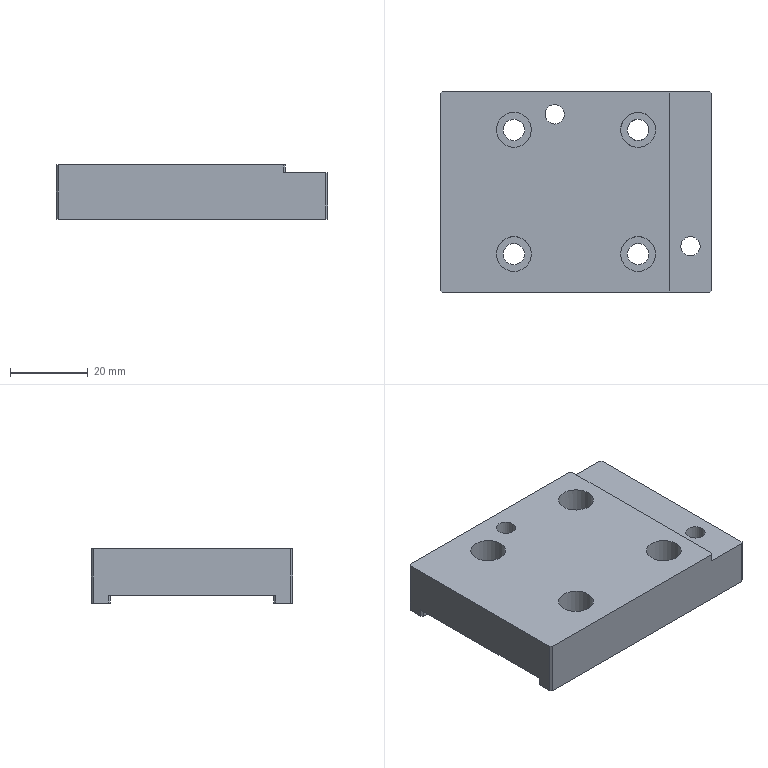Part | NX | 1 solid | 37 faces | box 70 x 52 x 14 mm | volume 41219 mm3 | plane 27 | cylinder 10 | commonest cylinder face diameters 5.5 x4 9 x4 5 x2
STEP:
#1=CARTESIAN_POINT('',(73.5,170.097,289.7));
#2=VERTEX_POINT('',#1);
#3=CARTESIAN_POINT('',(74.,170.597,289.7));
#4=VERTEX_POINT('',#3);
#5=CARTESIAN_POINT('',(69.25,165.847,289.7));
#6=DIRECTION('',(0.7071,0.7071,0.000000072));
#7=VECTOR('',#6,1000.);
#8=LINE('',#5,#7);
#9=EDGE_CURVE('',#2,#4,#8,.T.);
#10=ORIENTED_EDGE('',*,*,#9,.F.);
#11=CARTESIAN_POINT('',(4.5,170.097,289.7));
#12=VERTEX_POINT('',#11);
#13=CARTESIAN_POINT('',(39.,170.097,289.7));
#14=DIRECTION('',(-1.,0.,0.));
#15=VECTOR('',#14,1000.);
#16=LINE('',#13,#15);
#17=EDGE_CURVE('',#2,#12,#16,.T.);
#18=ORIENTED_EDGE('',*,*,#17,.T.);
#19=CARTESIAN_POINT('',(4.,170.597,289.7));
#20=VERTEX_POINT('',#19);
#21=CARTESIAN_POINT('',(8.75,165.847,289.7));
#22=DIRECTION('',(-0.7071,0.7071,0.000000072));
#23=VECTOR('',#22,1000.);
#24=LINE('',#21,#23);
#25=EDGE_CURVE('',#12,#20,#24,.T.);
#26=ORIENTED_EDGE('',*,*,#25,.T.);
#27=CARTESIAN_POINT('',(4.,174.557,289.7));
#28=VERTEX_POINT('',#27);
#29=CARTESIAN_POINT('',(4.,196.097,289.7));
#30=DIRECTION('',(0.,-1.,-0.000000102));
#31=VECTOR('',#30,1000.);
#32=LINE('',#29,#31);
#33=EDGE_CURVE('',#28,#20,#32,.T.);
#34=ORIENTED_EDGE('',*,*,#33,.F.);
#35=CARTESIAN_POINT('',(4.5,175.057,289.7));
#36=VERTEX_POINT('',#35);
#37=CARTESIAN_POINT('',(32.27,202.827,289.7));
#38=DIRECTION('',(-0.7071,-0.7071,-0.000000072));
#39=VECTOR('',#38,1000.);
#40=LINE('',#37,#39);
#41=EDGE_CURVE('',#36,#28,#40,.T.);
#42=ORIENTED_EDGE('',*,*,#41,.F.);
#43=CARTESIAN_POINT('',(73.5,175.057,289.7));
#44=VERTEX_POINT('',#43);
#45=CARTESIAN_POINT('',(39.,175.057,289.7));
#46=DIRECTION('',(-1.,0.,0.));
#47=VECTOR('',#46,1000.);
#48=LINE('',#45,#47);
#49=EDGE_CURVE('',#44,#36,#48,.T.);
#50=ORIENTED_EDGE('',*,*,#49,.F.);
#51=CARTESIAN_POINT('',(74.,174.557,289.7));
#52=VERTEX_POINT('',#51);
#53=CARTESIAN_POINT('',(45.73,202.827,289.7));
#54=DIRECTION('',(0.7071,-0.7071,-0.000000072));
#55=VECTOR('',#54,1000.);
#56=LINE('',#53,#55);
#57=EDGE_CURVE('',#44,#52,#56,.T.);
#58=ORIENTED_EDGE('',*,*,#57,.T.);
#59=CARTESIAN_POINT('',(74.,196.097,289.7));
#60=DIRECTION('',(0.,-1.,-0.000000102));
#61=VECTOR('',#60,1000.);
#62=LINE('',#59,#61);
#63=EDGE_CURVE('',#52,#4,#62,.T.);
#64=ORIENTED_EDGE('',*,*,#63,.T.);
#65=EDGE_LOOP('',(#10,#18,#26,#34,#42,#50,#58,#64));
#66=FACE_BOUND('',#65,.T.);
#67=CARTESIAN_POINT('',(39.,196.097,289.7));
#68=DIRECTION('',(0.,0.000000102,-1.));
#69=DIRECTION('',(-1.,0.,0.));
#70=AXIS2_PLACEMENT_3D('',#67,#68,#69);
#71=PLANE('',#70);
#72=ADVANCED_FACE('',(#66),#71,.T.);
#73=CARTESIAN_POINT('',(62.5,222.097,303.7));
#74=VERTEX_POINT('',#73);
#75=CARTESIAN_POINT('',(62.5,222.097,301.7));
#76=VERTEX_POINT('',#75);
#77=CARTESIAN_POINT('',(62.5,222.097,303.7));
#78=DIRECTION('',(0.,0.000000051,-1.));
#79=VECTOR('',#78,1000.);
#80=LINE('',#77,#79);
#81=EDGE_CURVE('',#74,#76,#80,.T.);
#82=ORIENTED_EDGE('',*,*,#81,.T.);
#83=CARTESIAN_POINT('',(73.5,222.097,301.7));
#84=VERTEX_POINT('',#83);
#85=CARTESIAN_POINT('',(68.25,222.097,301.7));
#86=DIRECTION('',(1.,0.,0.));
#87=VECTOR('',#86,1000.);
#88=LINE('',#85,#87);
#89=EDGE_CURVE('',#76,#84,#88,.T.);
#90=ORIENTED_EDGE('',*,*,#89,.T.);
#91=CARTESIAN_POINT('',(73.5,222.097,289.7));
#92=VERTEX_POINT('',#91);
#93=CARTESIAN_POINT('',(73.5,222.097,290.7));
#94=DIRECTION('',(0.,0.000000051,-1.));
#95=VECTOR('',#94,1000.);
#96=LINE('',#93,#95);
#97=EDGE_CURVE('',#84,#92,#96,.T.);
#98=ORIENTED_EDGE('',*,*,#97,.T.);
#99=CARTESIAN_POINT('',(4.5,222.097,289.7));
#100=VERTEX_POINT('',#99);
#101=CARTESIAN_POINT('',(39.,222.097,289.7));
#102=DIRECTION('',(1.,0.,0.));
#103=VECTOR('',#102,1000.);
#104=LINE('',#101,#103);
#105=EDGE_CURVE('',#92,#100,#104,.F.);
#106=ORIENTED_EDGE('',*,*,#105,.T.);
#107=CARTESIAN_POINT('',(4.5,222.097,303.7));
#108=VERTEX_POINT('',#107);
#109=CARTESIAN_POINT('',(4.5,222.097,290.7));
#110=DIRECTION('',(0.,-0.000000051,1.));
#111=VECTOR('',#110,1000.);
#112=LINE('',#109,#111);
#113=EDGE_CURVE('',#100,#108,#112,.T.);
#114=ORIENTED_EDGE('',*,*,#113,.T.);
#115=CARTESIAN_POINT('',(63.05,222.097,303.7));
#116=DIRECTION('',(1.,0.,0.));
#117=VECTOR('',#116,1000.);
#118=LINE('',#115,#117);
#119=EDGE_CURVE('',#108,#74,#118,.T.);
#120=ORIENTED_EDGE('',*,*,#119,.T.);
#121=EDGE_LOOP('',(#82,#90,#98,#106,#114,#120));
#122=FACE_BOUND('',#121,.T.);
#123=CARTESIAN_POINT('',(63.05,222.097,290.7));
#124=DIRECTION('',(0.,1.,0.000000051));
#125=DIRECTION('',(0.,-0.000000051,1.));
#126=AXIS2_PLACEMENT_3D('',#123,#124,#125);
#127=PLANE('',#126);
#128=ADVANCED_FACE('',(#122),#127,.T.);
#129=ORIENTED_EDGE('',*,*,#81,.F.);
#130=CARTESIAN_POINT('',(63.,221.597,303.7));
#131=VERTEX_POINT('',#130);
#132=CARTESIAN_POINT('',(62.5,222.097,303.7));
#133=DIRECTION('',(0.7071,-0.7071,-0.000000072));
#134=VECTOR('',#133,1000.);
#135=LINE('',#132,#134);
#136=EDGE_CURVE('',#74,#131,#135,.T.);
#137=ORIENTED_EDGE('',*,*,#136,.T.);
#138=CARTESIAN_POINT('',(63.,221.597,301.7));
#139=VERTEX_POINT('',#138);
#140=CARTESIAN_POINT('',(63.,221.597,301.7));
#141=DIRECTION('',(0.,-0.000000051,1.));
#142=VECTOR('',#141,1000.);
#143=LINE('',#140,#142);
#144=EDGE_CURVE('',#139,#131,#143,.T.);
#145=ORIENTED_EDGE('',*,*,#144,.F.);
#146=CARTESIAN_POINT('',(78.375,206.222,301.7));
#147=DIRECTION('',(0.7071,-0.7071,-0.000000072));
#148=VECTOR('',#147,1000.);
#149=LINE('',#146,#148);
#150=EDGE_CURVE('',#139,#76,#149,.F.);
#151=ORIENTED_EDGE('',*,*,#150,.T.);
#152=EDGE_LOOP('',(#129,#137,#145,#151));
#153=FACE_BOUND('',#152,.T.);
#154=CARTESIAN_POINT('',(62.5,222.097,290.7));
#155=DIRECTION('',(0.7071,0.7071,0.000000036));
#156=DIRECTION('',(0.,0.000000051,-1.));
#157=AXIS2_PLACEMENT_3D('',#154,#155,#156);
#158=PLANE('',#157);
#159=ADVANCED_FACE('',(#153),#158,.T.);
#160=CARTESIAN_POINT('',(63.,170.597,303.7));
#161=VERTEX_POINT('',#160);
#162=CARTESIAN_POINT('',(63.,-123.903,303.7));
#163=DIRECTION('',(0.,1.,0.000000102));
#164=VECTOR('',#163,1000.);
#165=LINE('',#162,#164);
#166=EDGE_CURVE('',#161,#131,#165,.T.);
#167=ORIENTED_EDGE('',*,*,#166,.F.);
#168=CARTESIAN_POINT('',(63.,170.597,301.7));
#169=VERTEX_POINT('',#168);
#170=CARTESIAN_POINT('',(63.,170.597,303.7));
#171=DIRECTION('',(0.,0.000000051,-1.));
#172=VECTOR('',#171,1000.);
#173=LINE('',#170,#172);
#174=EDGE_CURVE('',#161,#169,#173,.T.);
#175=ORIENTED_EDGE('',*,*,#174,.T.);
#176=CARTESIAN_POINT('',(63.,196.097,301.7));
#177=DIRECTION('',(0.,-1.,-0.000000102));
#178=VECTOR('',#177,1000.);
#179=LINE('',#176,#178);
#180=EDGE_CURVE('',#139,#169,#179,.T.);
#181=ORIENTED_EDGE('',*,*,#180,.F.);
#182=ORIENTED_EDGE('',*,*,#144,.T.);
#183=EDGE_LOOP('',(#167,#175,#181,#182));
#184=FACE_BOUND('',#183,.T.);
#185=CARTESIAN_POINT('',(63.,-123.903,301.7));
#186=DIRECTION('',(-1.,0.,0.));
#187=DIRECTION('',(0.,-0.000000051,1.));
#188=AXIS2_PLACEMENT_3D('',#185,#186,#187);
#189=PLANE('',#188);
#190=ADVANCED_FACE('',(#184),#189,.F.);
#191=ORIENTED_EDGE('',*,*,#174,.F.);
#192=CARTESIAN_POINT('',(62.5,170.097,303.7));
#193=VERTEX_POINT('',#192);
#194=CARTESIAN_POINT('',(63.,170.597,303.7));
#195=DIRECTION('',(-0.7071,-0.7071,-0.000000072));
#196=VECTOR('',#195,1000.);
#197=LINE('',#194,#196);
#198=EDGE_CURVE('',#161,#193,#197,.T.);
#199=ORIENTED_EDGE('',*,*,#198,.T.);
#200=CARTESIAN_POINT('',(62.5,170.097,301.7));
#201=VERTEX_POINT('',#200);
#202=CARTESIAN_POINT('',(62.5,170.097,301.7));
#203=DIRECTION('',(0.,-0.000000051,1.));
#204=VECTOR('',#203,1000.);
#205=LINE('',#202,#204);
#206=EDGE_CURVE('',#201,#193,#205,.T.);
#207=ORIENTED_EDGE('',*,*,#206,.F.);
#208=CARTESIAN_POINT('',(63.,170.597,301.7));
#209=DIRECTION('',(0.7071,0.7071,0.000000072));
#210=VECTOR('',#209,1000.);
#211=LINE('',#208,#210);
#212=EDGE_CURVE('',#169,#201,#211,.F.);
#213=ORIENTED_EDGE('',*,*,#212,.F.);
#214=EDGE_LOOP('',(#191,#199,#207,#213));
#215=FACE_BOUND('',#214,.T.);
#216=CARTESIAN_POINT('',(63.,170.597,301.7));
#217=DIRECTION('',(0.7071,-0.7071,-0.000000036));
#218=DIRECTION('',(0.,0.000000051,-1.));
#219=AXIS2_PLACEMENT_3D('',#216,#217,#218);
#220=PLANE('',#219);
#221=ADVANCED_FACE('',(#215),#220,.T.);
#222=ORIENTED_EDGE('',*,*,#17,.F.);
#223=CARTESIAN_POINT('',(73.5,170.097,301.7));
#224=VERTEX_POINT('',#223);
#225=CARTESIAN_POINT('',(73.5,170.097,284.2));
#226=DIRECTION('',(0.,-0.000000051,1.));
#227=VECTOR('',#226,1000.);
#228=LINE('',#225,#227);
#229=EDGE_CURVE('',#2,#224,#228,.T.);
#230=ORIENTED_EDGE('',*,*,#229,.T.);
#231=CARTESIAN_POINT('',(63.05,170.097,301.7));
#232=DIRECTION('',(1.,0.,0.));
#233=VECTOR('',#232,1000.);
#234=LINE('',#231,#233);
#235=EDGE_CURVE('',#201,#224,#234,.T.);
#236=ORIENTED_EDGE('',*,*,#235,.F.);
#237=ORIENTED_EDGE('',*,*,#206,.T.);
#238=CARTESIAN_POINT('',(4.5,170.097,303.7));
#239=VERTEX_POINT('',#238);
#240=CARTESIAN_POINT('',(63.05,170.097,303.7));
#241=DIRECTION('',(-1.,0.,0.));
#242=VECTOR('',#241,1000.);
#243=LINE('',#240,#242);
#244=EDGE_CURVE('',#193,#239,#243,.T.);
#245=ORIENTED_EDGE('',*,*,#244,.T.);
#246=CARTESIAN_POINT('',(4.5,170.097,284.2));
#247=DIRECTION('',(0.,0.000000051,-1.));
#248=VECTOR('',#247,1000.);
#249=LINE('',#246,#248);
#250=EDGE_CURVE('',#239,#12,#249,.T.);
#251=ORIENTED_EDGE('',*,*,#250,.T.);
#252=EDGE_LOOP('',(#222,#230,#236,#237,#245,#251));
#253=FACE_BOUND('',#252,.T.);
#254=CARTESIAN_POINT('',(63.05,170.097,284.2));
#255=DIRECTION('',(0.,-1.,-0.000000051));
#256=DIRECTION('',(0.,0.000000051,-1.));
#257=AXIS2_PLACEMENT_3D('',#254,#255,#256);
#258=PLANE('',#257);
#259=ADVANCED_FACE('',(#253),#258,.T.);
#260=ORIENTED_EDGE('',*,*,#25,.F.);
#261=ORIENTED_EDGE('',*,*,#250,.F.);
#262=CARTESIAN_POINT('',(4.,170.597,303.7));
#263=VERTEX_POINT('',#262);
#264=CARTESIAN_POINT('',(4.5,170.097,303.7));
#265=DIRECTION('',(-0.7071,0.7071,0.000000072));
#266=VECTOR('',#265,1000.);
#267=LINE('',#264,#266);
#268=EDGE_CURVE('',#239,#263,#267,.T.);
#269=ORIENTED_EDGE('',*,*,#268,.T.);
#270=CARTESIAN_POINT('',(4.,170.597,288.7));
#271=DIRECTION('',(0.,-0.000000051,1.));
#272=VECTOR('',#271,1000.);
#273=LINE('',#270,#272);
#274=EDGE_CURVE('',#20,#263,#273,.T.);
#275=ORIENTED_EDGE('',*,*,#274,.F.);
#276=EDGE_LOOP('',(#260,#261,#269,#275));
#277=FACE_BOUND('',#276,.T.);
#278=CARTESIAN_POINT('',(4.5,170.097,284.2));
#279=DIRECTION('',(-0.7071,-0.7071,-0.000000036));
#280=DIRECTION('',(0.,0.000000051,-1.));
#281=AXIS2_PLACEMENT_3D('',#278,#279,#280);
#282=PLANE('',#281);
#283=ADVANCED_FACE('',(#277),#282,.T.);
#284=CARTESIAN_POINT('',(4.,174.557,291.7));
#285=VERTEX_POINT('',#284);
#286=CARTESIAN_POINT('',(4.,174.557,291.7));
#287=DIRECTION('',(0.,0.000000051,-1.));
#288=VECTOR('',#287,1000.);
#289=LINE('',#286,#288);
#290=EDGE_CURVE('',#285,#28,#289,.T.);
#291=ORIENTED_EDGE('',*,*,#290,.T.);
#292=ORIENTED_EDGE('',*,*,#33,.T.);
#293=ORIENTED_EDGE('',*,*,#274,.T.);
#294=CARTESIAN_POINT('',(4.,221.597,303.7));
#295=VERTEX_POINT('',#294);
#296=CARTESIAN_POINT('',(4.,214.797,303.7));
#297=DIRECTION('',(0.,-1.,-0.000000102));
#298=VECTOR('',#297,1000.);
#299=LINE('',#296,#298);
#300=EDGE_CURVE('',#295,#263,#299,.T.);
#301=ORIENTED_EDGE('',*,*,#300,.F.);
#302=CARTESIAN_POINT('',(4.,221.597,289.7));
#303=VERTEX_POINT('',#302);
#304=CARTESIAN_POINT('',(4.,221.597,288.7));
#305=DIRECTION('',(0.,0.000000051,-1.));
#306=VECTOR('',#305,1000.);
#307=LINE('',#304,#306);
#308=EDGE_CURVE('',#295,#303,#307,.T.);
#309=ORIENTED_EDGE('',*,*,#308,.T.);
#310=CARTESIAN_POINT('',(4.,217.637,289.7));
#311=VERTEX_POINT('',#310);
#312=CARTESIAN_POINT('',(4.,214.797,289.7));
#313=DIRECTION('',(0.,1.,0.000000102));
#314=VECTOR('',#313,1000.);
#315=LINE('',#312,#314);
#316=EDGE_CURVE('',#311,#303,#315,.T.);
#317=ORIENTED_EDGE('',*,*,#316,.F.);
#318=CARTESIAN_POINT('',(4.,217.637,291.7));
#319=VERTEX_POINT('',#318);
#320=CARTESIAN_POINT('',(4.,217.637,289.7));
#321=DIRECTION('',(0.,-0.000000051,1.));
#322=VECTOR('',#321,1000.);
#323=LINE('',#320,#322);
#324=EDGE_CURVE('',#311,#319,#323,.T.);
#325=ORIENTED_EDGE('',*,*,#324,.T.);
#326=CARTESIAN_POINT('',(4.,214.797,291.7));
#327=DIRECTION('',(0.,1.,0.000000102));
#328=VECTOR('',#327,1000.);
#329=LINE('',#326,#328);
#330=EDGE_CURVE('',#285,#319,#329,.T.);
#331=ORIENTED_EDGE('',*,*,#330,.F.);
#332=EDGE_LOOP('',(#291,#292,#293,#301,#309,#317,#325,#331));
#333=FACE_BOUND('',#332,.T.);
#334=CARTESIAN_POINT('',(4.,214.797,288.7));
#335=DIRECTION('',(1.,0.,0.));
#336=DIRECTION('',(0.,-1.,-0.000000051));
#337=AXIS2_PLACEMENT_3D('',#334,#335,#336);
#338=PLANE('',#337);
#339=ADVANCED_FACE('',(#333),#338,.F.);
#340=ORIENTED_EDGE('',*,*,#308,.F.);
#341=CARTESIAN_POINT('',(4.,221.597,303.7));
#342=DIRECTION('',(0.7071,0.7071,0.000000072));
#343=VECTOR('',#342,1000.);
#344=LINE('',#341,#343);
#345=EDGE_CURVE('',#295,#108,#344,.T.);
#346=ORIENTED_EDGE('',*,*,#345,.T.);
#347=ORIENTED_EDGE('',*,*,#113,.F.);
#348=CARTESIAN_POINT('',(4.,221.597,289.7));
#349=DIRECTION('',(-0.7071,-0.7071,-0.000000072));
#350=VECTOR('',#349,1000.);
#351=LINE('',#348,#350);
#352=EDGE_CURVE('',#303,#100,#351,.F.);
#353=ORIENTED_EDGE('',*,*,#352,.F.);
#354=EDGE_LOOP('',(#340,#346,#347,#353));
#355=FACE_BOUND('',#354,.T.);
#356=CARTESIAN_POINT('',(4.,221.597,288.7));
#357=DIRECTION('',(-0.7071,0.7071,0.000000036));
#358=DIRECTION('',(0.,0.000000051,-1.));
#359=AXIS2_PLACEMENT_3D('',#356,#357,#358);
#360=PLANE('',#359);
#361=ADVANCED_FACE('',(#355),#360,.T.);
#362=ORIENTED_EDGE('',*,*,#57,.F.);
#363=CARTESIAN_POINT('',(73.5,175.057,291.7));
#364=VERTEX_POINT('',#363);
#365=CARTESIAN_POINT('',(73.5,175.057,291.7));
#366=DIRECTION('',(0.,0.000000051,-1.));
#367=VECTOR('',#366,1000.);
#368=LINE('',#365,#367);
#369=EDGE_CURVE('',#364,#44,#368,.T.);
#370=ORIENTED_EDGE('',*,*,#369,.F.);
#371=CARTESIAN_POINT('',(74.,174.557,291.7));
#372=VERTEX_POINT('',#371);
#373=CARTESIAN_POINT('',(45.73,202.827,291.7));
#374=DIRECTION('',(0.7071,-0.7071,-0.000000072));
#375=VECTOR('',#374,1000.);
#376=LINE('',#373,#375);
#377=EDGE_CURVE('',#364,#372,#376,.T.);
#378=ORIENTED_EDGE('',*,*,#377,.T.);
#379=CARTESIAN_POINT('',(74.,174.557,289.7));
#380=DIRECTION('',(0.,-0.000000051,1.));
#381=VECTOR('',#380,1000.);
#382=LINE('',#379,#381);
#383=EDGE_CURVE('',#52,#372,#382,.T.);
#384=ORIENTED_EDGE('',*,*,#383,.F.);
#385=EDGE_LOOP('',(#362,#370,#378,#384));
#386=FACE_BOUND('',#385,.T.);
#387=CARTESIAN_POINT('',(74.,174.557,288.7));
#388=DIRECTION('',(0.7071,0.7071,0.000000036));
#389=DIRECTION('',(0.,-0.000000051,1.));
#390=AXIS2_PLACEMENT_3D('',#387,#388,#389);
#391=PLANE('',#390);
#392=ADVANCED_FACE('',(#386),#391,.T.);
#393=ORIENTED_EDGE('',*,*,#229,.F.);
#394=ORIENTED_EDGE('',*,*,#9,.T.);
#395=CARTESIAN_POINT('',(74.,170.597,301.7));
#396=VERTEX_POINT('',#395);
#397=CARTESIAN_POINT('',(74.,170.597,288.7));
#398=DIRECTION('',(0.,0.000000051,-1.));
#399=VECTOR('',#398,1000.);
#400=LINE('',#397,#399);
#401=EDGE_CURVE('',#396,#4,#400,.T.);
#402=ORIENTED_EDGE('',*,*,#401,.F.);
#403=CARTESIAN_POINT('',(83.875,180.472,301.7));
#404=DIRECTION('',(0.7071,0.7071,0.000000072));
#405=VECTOR('',#404,1000.);
#406=LINE('',#403,#405);
#407=EDGE_CURVE('',#396,#224,#406,.F.);
#408=ORIENTED_EDGE('',*,*,#407,.T.);
#409=EDGE_LOOP('',(#393,#394,#402,#408));
#410=FACE_BOUND('',#409,.T.);
#411=CARTESIAN_POINT('',(74.,170.597,288.7));
#412=DIRECTION('',(-0.7071,0.7071,0.000000036));
#413=DIRECTION('',(0.,-0.000000051,1.));
#414=AXIS2_PLACEMENT_3D('',#411,#412,#413);
#415=PLANE('',#414);
#416=ADVANCED_FACE('',(#410),#415,.F.);
#417=CARTESIAN_POINT('',(73.5,217.137,289.7));
#418=VERTEX_POINT('',#417);
#419=CARTESIAN_POINT('',(73.5,217.137,291.7));
#420=VERTEX_POINT('',#419);
#421=CARTESIAN_POINT('',(73.5,217.137,289.7));
#422=DIRECTION('',(0.,-0.000000051,1.));
#423=VECTOR('',#422,1000.);
#424=LINE('',#421,#423);
#425=EDGE_CURVE('',#418,#420,#424,.T.);
#426=ORIENTED_EDGE('',*,*,#425,.F.);
#427=CARTESIAN_POINT('',(74.,217.637,289.7));
#428=VERTEX_POINT('',#427);
#429=CARTESIAN_POINT('',(45.73,189.367,289.7));
#430=DIRECTION('',(-0.7071,-0.7071,-0.000000072));
#431=VECTOR('',#430,1000.);
#432=LINE('',#429,#431);
#433=EDGE_CURVE('',#418,#428,#432,.F.);
#434=ORIENTED_EDGE('',*,*,#433,.T.);
#435=CARTESIAN_POINT('',(74.,217.637,291.7));
#436=VERTEX_POINT('',#435);
#437=CARTESIAN_POINT('',(74.,217.637,291.7));
#438=DIRECTION('',(0.,0.000000051,-1.));
#439=VECTOR('',#438,1000.);
#440=LINE('',#437,#439);
#441=EDGE_CURVE('',#436,#428,#440,.T.);
#442=ORIENTED_EDGE('',*,*,#441,.F.);
#443=CARTESIAN_POINT('',(45.73,189.367,291.7));
#444=DIRECTION('',(-0.7071,-0.7071,-0.000000072));
#445=VECTOR('',#444,1000.);
#446=LINE('',#443,#445);
#447=EDGE_CURVE('',#436,#420,#446,.T.);
#448=ORIENTED_EDGE('',*,*,#447,.T.);
#449=EDGE_LOOP('',(#426,#434,#442,#448));
#450=FACE_BOUND('',#449,.T.);
#451=CARTESIAN_POINT('',(74.,217.637,288.7));
#452=DIRECTION('',(0.7071,-0.7071,-0.000000036));
#453=DIRECTION('',(0.,0.000000051,-1.));
#454=AXIS2_PLACEMENT_3D('',#451,#452,#453);
#455=PLANE('',#454);
#456=ADVANCED_FACE('',(#450),#455,.T.);
#457=CARTESIAN_POINT('',(4.5,175.057,291.7));
#458=VERTEX_POINT('',#457);
#459=CARTESIAN_POINT('',(4.5,175.057,289.7));
#460=DIRECTION('',(0.,-0.000000051,1.));
#461=VECTOR('',#460,1000.);
#462=LINE('',#459,#461);
#463=EDGE_CURVE('',#36,#458,#462,.T.);
#464=ORIENTED_EDGE('',*,*,#463,.F.);
#465=ORIENTED_EDGE('',*,*,#41,.T.);
#466=ORIENTED_EDGE('',*,*,#290,.F.);
#467=CARTESIAN_POINT('',(4.,174.557,291.7));
#468=DIRECTION('',(0.7071,0.7071,0.000000072));
#469=VECTOR('',#468,1000.);
#470=LINE('',#467,#469);
#471=EDGE_CURVE('',#458,#285,#470,.F.);
#472=ORIENTED_EDGE('',*,*,#471,.F.);
#473=EDGE_LOOP('',(#464,#465,#466,#472));
#474=FACE_BOUND('',#473,.T.);
#475=CARTESIAN_POINT('',(4.,174.557,288.7));
#476=DIRECTION('',(0.7071,-0.7071,-0.000000036));
#477=DIRECTION('',(0.,-0.000000051,1.));
#478=AXIS2_PLACEMENT_3D('',#475,#476,#477);
#479=PLANE('',#478);
#480=ADVANCED_FACE('',(#474),#479,.F.);
#481=ORIENTED_EDGE('',*,*,#324,.F.);
#482=CARTESIAN_POINT('',(4.5,217.137,289.7));
#483=VERTEX_POINT('',#482);
#484=CARTESIAN_POINT('',(4.,217.637,289.7));
#485=DIRECTION('',(-0.7071,0.7071,0.000000072));
#486=VECTOR('',#485,1000.);
#487=LINE('',#484,#486);
#488=EDGE_CURVE('',#483,#311,#487,.T.);
#489=ORIENTED_EDGE('',*,*,#488,.F.);
#490=CARTESIAN_POINT('',(4.5,217.137,291.7));
#491=VERTEX_POINT('',#490);
#492=CARTESIAN_POINT('',(4.5,217.137,291.7));
#493=DIRECTION('',(0.,0.000000051,-1.));
#494=VECTOR('',#493,1000.);
#495=LINE('',#492,#494);
#496=EDGE_CURVE('',#491,#483,#495,.T.);
#497=ORIENTED_EDGE('',*,*,#496,.F.);
#498=CARTESIAN_POINT('',(32.27,189.367,291.7));
#499=DIRECTION('',(0.7071,-0.7071,-0.000000072));
#500=VECTOR('',#499,1000.);
#501=LINE('',#498,#500);
#502=EDGE_CURVE('',#491,#319,#501,.F.);
#503=ORIENTED_EDGE('',*,*,#502,.T.);
#504=EDGE_LOOP('',(#481,#489,#497,#503));
#505=FACE_BOUND('',#504,.T.);
#506=CARTESIAN_POINT('',(4.,217.637,288.7));
#507=DIRECTION('',(0.7071,0.7071,0.000000036));
#508=DIRECTION('',(0.,0.000000051,-1.));
#509=AXIS2_PLACEMENT_3D('',#506,#507,#508);
#510=PLANE('',#509);
#511=ADVANCED_FACE('',(#505),#510,.F.);
#512=CARTESIAN_POINT('',(74.,221.597,289.7));
#513=VERTEX_POINT('',#512);
#514=CARTESIAN_POINT('',(74.,221.597,301.7));
#515=VERTEX_POINT('',#514);
#516=CARTESIAN_POINT('',(74.,221.597,288.7));
#517=DIRECTION('',(0.,-0.000000051,1.));
#518=VECTOR('',#517,1000.);
#519=LINE('',#516,#518);
#520=EDGE_CURVE('',#513,#515,#519,.T.);
#521=ORIENTED_EDGE('',*,*,#520,.F.);
#522=CARTESIAN_POINT('',(69.25,226.347,289.7));
#523=DIRECTION('',(-0.7071,0.7071,0.000000072));
#524=VECTOR('',#523,1000.);
#525=LINE('',#522,#524);
#526=EDGE_CURVE('',#513,#92,#525,.T.);
#527=ORIENTED_EDGE('',*,*,#526,.T.);
#528=ORIENTED_EDGE('',*,*,#97,.F.);
#529=CARTESIAN_POINT('',(83.875,211.722,301.7));
#530=DIRECTION('',(-0.7071,0.7071,0.000000072));
#531=VECTOR('',#530,1000.);
#532=LINE('',#529,#531);
#533=EDGE_CURVE('',#84,#515,#532,.F.);
#534=ORIENTED_EDGE('',*,*,#533,.T.);
#535=EDGE_LOOP('',(#521,#527,#528,#534));
#536=FACE_BOUND('',#535,.T.);
#537=CARTESIAN_POINT('',(73.5,222.097,290.7));
#538=DIRECTION('',(-0.7071,-0.7071,-0.000000036));
#539=DIRECTION('',(0.,-0.000000051,1.));
#540=AXIS2_PLACEMENT_3D('',#537,#538,#539);
#541=PLANE('',#540);
#542=ADVANCED_FACE('',(#536),#541,.F.);
#543=CARTESIAN_POINT('',(68.5,184.597,301.7));
#544=VERTEX_POINT('',#543);
#545=CARTESIAN_POINT('',(68.5,182.097,301.7));
#546=DIRECTION('',(0.,0.000000102,-1.));
#547=DIRECTION('',(0.,1.,0.000000102));
#548=AXIS2_PLACEMENT_3D('',#545,#546,#547);
#549=CIRCLE('',#548,2.5);
#550=EDGE_CURVE('',#544,#544,#549,.T.);
#551=ORIENTED_EDGE('',*,*,#550,.F.);
#552=EDGE_LOOP('',(#551));
#553=FACE_BOUND('',#552,.T.);
#554=CARTESIAN_POINT('',(68.5,184.597,291.7));
#555=VERTEX_POINT('',#554);
#556=CARTESIAN_POINT('',(68.5,182.097,291.7));
#557=DIRECTION('',(0.,0.000000102,-1.));
#558=DIRECTION('',(0.,1.,0.000000102));
#559=AXIS2_PLACEMENT_3D('',#556,#557,#558);
#560=CIRCLE('',#559,2.5);
#561=EDGE_CURVE('',#555,#555,#560,.T.);
#562=ORIENTED_EDGE('',*,*,#561,.T.);
#563=EDGE_LOOP('',(#562));
#564=FACE_BOUND('',#563,.T.);
#565=CARTESIAN_POINT('',(68.5,182.097,301.7));
#566=DIRECTION('',(0.,0.000000102,-1.));
#567=DIRECTION('',(1.,0.,0.));
#568=AXIS2_PLACEMENT_3D('',#565,#566,#567);
#569=CYLINDRICAL_SURFACE('',#568,2.5);
#570=ADVANCED_FACE('',(#553,#564),#569,.F.);
#571=CARTESIAN_POINT('',(33.5,213.597,303.7));
#572=VERTEX_POINT('',#571);
#573=CARTESIAN_POINT('',(33.5,216.097,303.7));
#574=DIRECTION('',(0.,0.000000102,-1.));
#575=DIRECTION('',(0.,-1.,-0.000000102));
#576=AXIS2_PLACEMENT_3D('',#573,#574,#575);
#577=CIRCLE('',#576,2.5);
#578=EDGE_CURVE('',#572,#572,#577,.T.);
#579=ORIENTED_EDGE('',*,*,#578,.F.);
#580=EDGE_LOOP('',(#579));
#581=FACE_BOUND('',#580,.T.);
#582=CARTESIAN_POINT('',(35.773,217.137,291.7));
#583=VERTEX_POINT('',#582);
#584=CARTESIAN_POINT('',(35.773,217.137,289.7));
#585=VERTEX_POINT('',#584);
#586=CARTESIAN_POINT('',(35.773,217.137,291.7));
#587=CARTESIAN_POINT('',(35.773,217.137,291.45));
#588=CARTESIAN_POINT('',(35.773,217.137,291.2));
#589=CARTESIAN_POINT('',(35.773,217.137,290.95));
#590=CARTESIAN_POINT('',(35.773,217.137,290.7));
#591=CARTESIAN_POINT('',(35.773,217.137,290.45));
#592=CARTESIAN_POINT('',(35.773,217.137,290.2));
#593=CARTESIAN_POINT('',(35.773,217.137,290.033));
#594=CARTESIAN_POINT('',(35.773,217.137,289.867));
#595=CARTESIAN_POINT('',(35.773,217.137,289.7));
#596=B_SPLINE_CURVE_WITH_KNOTS('',3,(#586,#587,#588,#589,#590,#591,#592,#593,#594,#595),.UNSPECIFIED.,.F.,.F.,(4,3,3,4),(0.,0.5,1.,1.333),.PIECEWISE_BEZIER_KNOTS.);
#597=EDGE_CURVE('',#583,#585,#596,.T.);
#598=ORIENTED_EDGE('',*,*,#597,.F.);
#599=CARTESIAN_POINT('',(31.227,217.137,291.7));
#600=VERTEX_POINT('',#599);
#601=CARTESIAN_POINT('',(33.5,216.097,291.7));
#602=DIRECTION('',(0.,0.000000102,-1.));
#603=DIRECTION('',(0.,1.,0.000000102));
#604=AXIS2_PLACEMENT_3D('',#601,#602,#603);
#605=CIRCLE('',#604,2.5);
#606=EDGE_CURVE('',#583,#600,#605,.T.);
#607=ORIENTED_EDGE('',*,*,#606,.T.);
#608=CARTESIAN_POINT('',(31.227,217.137,289.7));
#609=VERTEX_POINT('',#608);
#610=CARTESIAN_POINT('',(31.227,217.137,289.7));
#611=CARTESIAN_POINT('',(31.227,217.137,289.867));
#612=CARTESIAN_POINT('',(31.227,217.137,290.033));
#613=CARTESIAN_POINT('',(31.227,217.137,290.2));
#614=CARTESIAN_POINT('',(31.227,217.137,290.45));
#615=CARTESIAN_POINT('',(31.227,217.137,290.7));
#616=CARTESIAN_POINT('',(31.227,217.137,290.95));
#617=CARTESIAN_POINT('',(31.227,217.137,291.2));
#618=CARTESIAN_POINT('',(31.227,217.137,291.45));
#619=CARTESIAN_POINT('',(31.227,217.137,291.7));
#620=B_SPLINE_CURVE_WITH_KNOTS('',3,(#610,#611,#612,#613,#614,#615,#616,#617,#618,#619),.UNSPECIFIED.,.F.,.F.,(4,3,3,4),(-0.3333,0.,0.5,1.),.PIECEWISE_BEZIER_KNOTS.);
#621=EDGE_CURVE('',#609,#600,#620,.T.);
#622=ORIENTED_EDGE('',*,*,#621,.F.);
#623=CARTESIAN_POINT('',(33.5,216.097,289.7));
#624=DIRECTION('',(0.,0.000000102,-1.));
#625=DIRECTION('',(0.,1.,0.000000102));
#626=AXIS2_PLACEMENT_3D('',#623,#624,#625);
#627=CIRCLE('',#626,2.5);
#628=EDGE_CURVE('',#609,#585,#627,.T.);
#629=ORIENTED_EDGE('',*,*,#628,.T.);
#630=EDGE_LOOP('',(#598,#607,#622,#629));
#631=FACE_BOUND('',#630,.T.);
#632=CARTESIAN_POINT('',(33.5,216.097,303.7));
#633=DIRECTION('',(0.,0.000000102,-1.));
#634=DIRECTION('',(1.,0.,0.));
#635=AXIS2_PLACEMENT_3D('',#632,#633,#634);
#636=CYLINDRICAL_SURFACE('',#635,2.5);
#637=ADVANCED_FACE('',(#581,#631),#636,.F.);
#638=ORIENTED_EDGE('',*,*,#150,.F.);
#639=ORIENTED_EDGE('',*,*,#180,.T.);
#640=ORIENTED_EDGE('',*,*,#212,.T.);
#641=ORIENTED_EDGE('',*,*,#235,.T.);
#642=ORIENTED_EDGE('',*,*,#407,.F.);
#643=CARTESIAN_POINT('',(74.,196.097,301.7));
#644=DIRECTION('',(0.,-1.,-0.000000102));
#645=VECTOR('',#644,1000.);
#646=LINE('',#643,#645);
#647=EDGE_CURVE('',#515,#396,#646,.T.);
#648=ORIENTED_EDGE('',*,*,#647,.F.);
#649=ORIENTED_EDGE('',*,*,#533,.F.);
#650=ORIENTED_EDGE('',*,*,#89,.F.);
#651=EDGE_LOOP('',(#638,#639,#640,#641,#642,#648,#649,#650));
#652=FACE_BOUND('',#651,.T.);
#653=ORIENTED_EDGE('',*,*,#550,.T.);
#654=EDGE_LOOP('',(#653));
#655=FACE_BOUND('',#654,.T.);
#656=CARTESIAN_POINT('',(68.25,196.097,301.7));
#657=DIRECTION('',(0.,0.000000102,-1.));
#658=DIRECTION('',(-1.,0.,0.));
#659=AXIS2_PLACEMENT_3D('',#656,#657,#658);
#660=PLANE('',#659);
#661=ADVANCED_FACE('',(#652,#655),#660,.F.);
#662=CARTESIAN_POINT('',(59.5,212.097,296.7));
#663=VERTEX_POINT('',#662);
#664=CARTESIAN_POINT('',(55.,212.097,296.7));
#665=DIRECTION('',(0.,0.000000102,-1.));
#666=DIRECTION('',(1.,0.,0.));
#667=AXIS2_PLACEMENT_3D('',#664,#665,#666);
#668=CIRCLE('',#667,4.5);
#669=EDGE_CURVE('',#663,#663,#668,.T.);
#670=ORIENTED_EDGE('',*,*,#669,.T.);
#671=EDGE_LOOP('',(#670));
#672=FACE_BOUND('',#671,.T.);
#673=CARTESIAN_POINT('',(55.,207.597,303.7));
#674=VERTEX_POINT('',#673);
#675=CARTESIAN_POINT('',(55.,212.097,303.7));
#676=DIRECTION('',(0.,-0.000000102,1.));
#677=DIRECTION('',(0.,-1.,-0.000000102));
#678=AXIS2_PLACEMENT_3D('',#675,#676,#677);
#679=CIRCLE('',#678,4.5);
#680=EDGE_CURVE('',#674,#674,#679,.T.);
#681=ORIENTED_EDGE('',*,*,#680,.T.);
#682=EDGE_LOOP('',(#681));
#683=FACE_BOUND('',#682,.T.);
#684=CARTESIAN_POINT('',(55.,212.097,303.7));
#685=DIRECTION('',(0.,0.000000102,-1.));
#686=DIRECTION('',(1.,0.,0.));
#687=AXIS2_PLACEMENT_3D('',#684,#685,#686);
#688=CYLINDRICAL_SURFACE('',#687,4.5);
#689=ADVANCED_FACE('',(#672,#683),#688,.F.);
#690=CARTESIAN_POINT('',(52.25,212.097,296.7));
#691=VERTEX_POINT('',#690);
#692=CARTESIAN_POINT('',(55.,212.097,296.7));
#693=DIRECTION('',(0.,-0.000000102,1.));
#694=DIRECTION('',(-1.,0.,0.));
#695=AXIS2_PLACEMENT_3D('',#692,#693,#694);
#696=CIRCLE('',#695,2.75);
#697=EDGE_CURVE('',#691,#691,#696,.T.);
#698=ORIENTED_EDGE('',*,*,#697,.F.);
#699=EDGE_LOOP('',(#698));
#700=FACE_BOUND('',#699,.T.);
#701=ORIENTED_EDGE('',*,*,#669,.F.);
#702=EDGE_LOOP('',(#701));
#703=FACE_BOUND('',#702,.T.);
#704=CARTESIAN_POINT('',(55.,212.097,296.7));
#705=DIRECTION('',(0.,0.000000102,-1.));
#706=DIRECTION('',(-1.,0.,0.));
#707=AXIS2_PLACEMENT_3D('',#704,#705,#706);
#708=PLANE('',#707);
#709=ADVANCED_FACE('',(#700,#703),#708,.F.);
#710=CARTESIAN_POINT('',(55.,184.597,296.7));
#711=VERTEX_POINT('',#710);
#712=CARTESIAN_POINT('',(55.,180.097,296.7));
#713=DIRECTION('',(0.,0.000000102,-1.));
#714=DIRECTION('',(0.,1.,0.000000102));
#715=AXIS2_PLACEMENT_3D('',#712,#713,#714);
#716=CIRCLE('',#715,4.5);
#717=EDGE_CURVE('',#711,#711,#716,.T.);
#718=ORIENTED_EDGE('',*,*,#717,.T.);
#719=EDGE_LOOP('',(#718));
#720=FACE_BOUND('',#719,.T.);
#721=CARTESIAN_POINT('',(55.,175.597,303.7));
#722=VERTEX_POINT('',#721);
#723=CARTESIAN_POINT('',(55.,180.097,303.7));
#724=DIRECTION('',(0.,-0.000000102,1.));
#725=DIRECTION('',(0.,-1.,-0.000000102));
#726=AXIS2_PLACEMENT_3D('',#723,#724,#725);
#727=CIRCLE('',#726,4.5);
#728=EDGE_CURVE('',#722,#722,#727,.T.);
#729=ORIENTED_EDGE('',*,*,#728,.T.);
#730=EDGE_LOOP('',(#729));
#731=FACE_BOUND('',#730,.T.);
#732=CARTESIAN_POINT('',(55.,180.097,303.7));
#733=DIRECTION('',(0.,0.000000102,-1.));
#734=DIRECTION('',(1.,0.,0.));
#735=AXIS2_PLACEMENT_3D('',#732,#733,#734);
#736=CYLINDRICAL_SURFACE('',#735,4.5);
#737=ADVANCED_FACE('',(#720,#731),#736,.F.);
#738=CARTESIAN_POINT('',(55.,182.847,296.7));
#739=VERTEX_POINT('',#738);
#740=CARTESIAN_POINT('',(55.,180.097,296.7));
#741=DIRECTION('',(0.,-0.000000102,1.));
#742=DIRECTION('',(0.,1.,0.000000102));
#743=AXIS2_PLACEMENT_3D('',#740,#741,#742);
#744=CIRCLE('',#743,2.75);
#745=EDGE_CURVE('',#739,#739,#744,.T.);
#746=ORIENTED_EDGE('',*,*,#745,.F.);
#747=EDGE_LOOP('',(#746));
#748=FACE_BOUND('',#747,.T.);
#749=ORIENTED_EDGE('',*,*,#717,.F.);
#750=EDGE_LOOP('',(#749));
#751=FACE_BOUND('',#750,.T.);
#752=CARTESIAN_POINT('',(55.,212.097,296.7));
#753=DIRECTION('',(0.,0.000000102,-1.));
#754=DIRECTION('',(-1.,0.,0.));
#755=AXIS2_PLACEMENT_3D('',#752,#753,#754);
#756=PLANE('',#755);
#757=ADVANCED_FACE('',(#748,#751),#756,.F.);
#758=CARTESIAN_POINT('',(23.,184.597,296.7));
#759=VERTEX_POINT('',#758);
#760=CARTESIAN_POINT('',(23.,180.097,296.7));
#761=DIRECTION('',(0.,0.000000102,-1.));
#762=DIRECTION('',(0.,1.,0.000000102));
#763=AXIS2_PLACEMENT_3D('',#760,#761,#762);
#764=CIRCLE('',#763,4.5);
#765=EDGE_CURVE('',#759,#759,#764,.T.);
#766=ORIENTED_EDGE('',*,*,#765,.T.);
#767=EDGE_LOOP('',(#766));
#768=FACE_BOUND('',#767,.T.);
#769=CARTESIAN_POINT('',(23.,175.597,303.7));
#770=VERTEX_POINT('',#769);
#771=CARTESIAN_POINT('',(23.,180.097,303.7));
#772=DIRECTION('',(0.,-0.000000102,1.));
#773=DIRECTION('',(0.,-1.,-0.000000102));
#774=AXIS2_PLACEMENT_3D('',#771,#772,#773);
#775=CIRCLE('',#774,4.5);
#776=EDGE_CURVE('',#770,#770,#775,.T.);
#777=ORIENTED_EDGE('',*,*,#776,.T.);
#778=EDGE_LOOP('',(#777));
#779=FACE_BOUND('',#778,.T.);
#780=CARTESIAN_POINT('',(23.,180.097,303.7));
#781=DIRECTION('',(0.,0.000000102,-1.));
#782=DIRECTION('',(1.,0.,0.));
#783=AXIS2_PLACEMENT_3D('',#780,#781,#782);
#784=CYLINDRICAL_SURFACE('',#783,4.5);
#785=ADVANCED_FACE('',(#768,#779),#784,.F.);
#786=CARTESIAN_POINT('',(23.,182.847,296.7));
#787=VERTEX_POINT('',#786);
#788=CARTESIAN_POINT('',(23.,180.097,296.7));
#789=DIRECTION('',(0.,-0.000000102,1.));
#790=DIRECTION('',(0.,1.,0.000000102));
#791=AXIS2_PLACEMENT_3D('',#788,#789,#790);
#792=CIRCLE('',#791,2.75);
#793=EDGE_CURVE('',#787,#787,#792,.T.);
#794=ORIENTED_EDGE('',*,*,#793,.F.);
#795=EDGE_LOOP('',(#794));
#796=FACE_BOUND('',#795,.T.);
#797=ORIENTED_EDGE('',*,*,#765,.F.);
#798=EDGE_LOOP('',(#797));
#799=FACE_BOUND('',#798,.T.);
#800=CARTESIAN_POINT('',(55.,212.097,296.7));
#801=DIRECTION('',(0.,0.000000102,-1.));
#802=DIRECTION('',(-1.,0.,0.));
#803=AXIS2_PLACEMENT_3D('',#800,#801,#802);
#804=PLANE('',#803);
#805=ADVANCED_FACE('',(#796,#799),#804,.F.);
#806=CARTESIAN_POINT('',(23.,216.597,296.7));
#807=VERTEX_POINT('',#806);
#808=CARTESIAN_POINT('',(23.,212.097,296.7));
#809=DIRECTION('',(0.,0.000000102,-1.));
#810=DIRECTION('',(0.,1.,0.000000102));
#811=AXIS2_PLACEMENT_3D('',#808,#809,#810);
#812=CIRCLE('',#811,4.5);
#813=EDGE_CURVE('',#807,#807,#812,.T.);
#814=ORIENTED_EDGE('',*,*,#813,.T.);
#815=EDGE_LOOP('',(#814));
#816=FACE_BOUND('',#815,.T.);
#817=CARTESIAN_POINT('',(23.,207.597,303.7));
#818=VERTEX_POINT('',#817);
#819=CARTESIAN_POINT('',(23.,212.097,303.7));
#820=DIRECTION('',(0.,-0.000000102,1.));
#821=DIRECTION('',(0.,-1.,-0.000000102));
#822=AXIS2_PLACEMENT_3D('',#819,#820,#821);
#823=CIRCLE('',#822,4.5);
#824=EDGE_CURVE('',#818,#818,#823,.T.);
#825=ORIENTED_EDGE('',*,*,#824,.T.);
#826=EDGE_LOOP('',(#825));
#827=FACE_BOUND('',#826,.T.);
#828=CARTESIAN_POINT('',(23.,212.097,303.7));
#829=DIRECTION('',(0.,0.000000102,-1.));
#830=DIRECTION('',(1.,0.,0.));
#831=AXIS2_PLACEMENT_3D('',#828,#829,#830);
#832=CYLINDRICAL_SURFACE('',#831,4.5);
#833=ADVANCED_FACE('',(#816,#827),#832,.F.);
#834=CARTESIAN_POINT('',(23.,214.847,296.7));
#835=VERTEX_POINT('',#834);
#836=CARTESIAN_POINT('',(23.,212.097,296.7));
#837=DIRECTION('',(0.,-0.000000102,1.));
#838=DIRECTION('',(0.,1.,0.000000102));
#839=AXIS2_PLACEMENT_3D('',#836,#837,#838);
#840=CIRCLE('',#839,2.75);
#841=EDGE_CURVE('',#835,#835,#840,.T.);
#842=ORIENTED_EDGE('',*,*,#841,.F.);
#843=EDGE_LOOP('',(#842));
#844=FACE_BOUND('',#843,.T.);
#845=ORIENTED_EDGE('',*,*,#813,.F.);
#846=EDGE_LOOP('',(#845));
#847=FACE_BOUND('',#846,.T.);
#848=CARTESIAN_POINT('',(55.,212.097,296.7));
#849=DIRECTION('',(0.,0.000000102,-1.));
#850=DIRECTION('',(-1.,0.,0.));
#851=AXIS2_PLACEMENT_3D('',#848,#849,#850);
#852=PLANE('',#851);
#853=ADVANCED_FACE('',(#844,#847),#852,.F.);
#854=CARTESIAN_POINT('',(55.,182.847,291.7));
#855=VERTEX_POINT('',#854);
#856=CARTESIAN_POINT('',(55.,180.097,291.7));
#857=DIRECTION('',(0.,-0.000000102,1.));
#858=DIRECTION('',(0.,1.,0.000000102));
#859=AXIS2_PLACEMENT_3D('',#856,#857,#858);
#860=CIRCLE('',#859,2.75);
#861=EDGE_CURVE('',#855,#855,#860,.T.);
#862=ORIENTED_EDGE('',*,*,#861,.F.);
#863=EDGE_LOOP('',(#862));
#864=FACE_BOUND('',#863,.T.);
#865=ORIENTED_EDGE('',*,*,#745,.T.);
#866=EDGE_LOOP('',(#865));
#867=FACE_BOUND('',#866,.T.);
#868=CARTESIAN_POINT('',(55.,180.097,289.7));
#869=DIRECTION('',(0.,-0.000000102,1.));
#870=DIRECTION('',(1.,0.,0.));
#871=AXIS2_PLACEMENT_3D('',#868,#869,#870);
#872=CYLINDRICAL_SURFACE('',#871,2.75);
#873=ADVANCED_FACE('',(#864,#867),#872,.F.);
#874=CARTESIAN_POINT('',(55.,214.847,291.7));
#875=VERTEX_POINT('',#874);
#876=CARTESIAN_POINT('',(55.,212.097,291.7));
#877=DIRECTION('',(0.,-0.000000102,1.));
#878=DIRECTION('',(0.,1.,0.000000102));
#879=AXIS2_PLACEMENT_3D('',#876,#877,#878);
#880=CIRCLE('',#879,2.75);
#881=EDGE_CURVE('',#875,#875,#880,.T.);
#882=ORIENTED_EDGE('',*,*,#881,.F.);
#883=EDGE_LOOP('',(#882));
#884=FACE_BOUND('',#883,.T.);
#885=ORIENTED_EDGE('',*,*,#697,.T.);
#886=EDGE_LOOP('',(#885));
#887=FACE_BOUND('',#886,.T.);
#888=CARTESIAN_POINT('',(55.,212.097,289.7));
#889=DIRECTION('',(0.,-0.000000102,1.));
#890=DIRECTION('',(1.,0.,0.));
#891=AXIS2_PLACEMENT_3D('',#888,#889,#890);
#892=CYLINDRICAL_SURFACE('',#891,2.75);
#893=ADVANCED_FACE('',(#884,#887),#892,.F.);
#894=CARTESIAN_POINT('',(23.,214.847,291.7));
#895=VERTEX_POINT('',#894);
#896=CARTESIAN_POINT('',(23.,212.097,291.7));
#897=DIRECTION('',(0.,-0.000000102,1.));
#898=DIRECTION('',(0.,1.,0.000000102));
#899=AXIS2_PLACEMENT_3D('',#896,#897,#898);
#900=CIRCLE('',#899,2.75);
#901=EDGE_CURVE('',#895,#895,#900,.T.);
#902=ORIENTED_EDGE('',*,*,#901,.F.);
#903=EDGE_LOOP('',(#902));
#904=FACE_BOUND('',#903,.T.);
#905=ORIENTED_EDGE('',*,*,#841,.T.);
#906=EDGE_LOOP('',(#905));
#907=FACE_BOUND('',#906,.T.);
#908=CARTESIAN_POINT('',(23.,212.097,289.7));
#909=DIRECTION('',(0.,-0.000000102,1.));
#910=DIRECTION('',(1.,0.,0.));
#911=AXIS2_PLACEMENT_3D('',#908,#909,#910);
#912=CYLINDRICAL_SURFACE('',#911,2.75);
#913=ADVANCED_FACE('',(#904,#907),#912,.F.);
#914=CARTESIAN_POINT('',(23.,182.847,291.7));
#915=VERTEX_POINT('',#914);
#916=CARTESIAN_POINT('',(23.,180.097,291.7));
#917=DIRECTION('',(0.,-0.000000102,1.));
#918=DIRECTION('',(0.,1.,0.000000102));
#919=AXIS2_PLACEMENT_3D('',#916,#917,#918);
#920=CIRCLE('',#919,2.75);
#921=EDGE_CURVE('',#915,#915,#920,.T.);
#922=ORIENTED_EDGE('',*,*,#921,.F.);
#923=EDGE_LOOP('',(#922));
#924=FACE_BOUND('',#923,.T.);
#925=ORIENTED_EDGE('',*,*,#793,.T.);
#926=EDGE_LOOP('',(#925));
#927=FACE_BOUND('',#926,.T.);
#928=CARTESIAN_POINT('',(23.,180.097,289.7));
#929=DIRECTION('',(0.,-0.000000102,1.));
#930=DIRECTION('',(1.,0.,0.));
#931=AXIS2_PLACEMENT_3D('',#928,#929,#930);
#932=CYLINDRICAL_SURFACE('',#931,2.75);
#933=ADVANCED_FACE('',(#924,#927),#932,.F.);
#934=ORIENTED_EDGE('',*,*,#921,.T.);
#935=EDGE_LOOP('',(#934));
#936=FACE_BOUND('',#935,.T.);
#937=ORIENTED_EDGE('',*,*,#861,.T.);
#938=EDGE_LOOP('',(#937));
#939=FACE_BOUND('',#938,.T.);
#940=ORIENTED_EDGE('',*,*,#901,.T.);
#941=EDGE_LOOP('',(#940));
#942=FACE_BOUND('',#941,.T.);
#943=ORIENTED_EDGE('',*,*,#881,.T.);
#944=EDGE_LOOP('',(#943));
#945=FACE_BOUND('',#944,.T.);
#946=CARTESIAN_POINT('',(39.,175.057,291.7));
#947=DIRECTION('',(-1.,0.,0.));
#948=VECTOR('',#947,1000.);
#949=LINE('',#946,#948);
#950=EDGE_CURVE('',#364,#458,#949,.T.);
#951=ORIENTED_EDGE('',*,*,#950,.T.);
#952=ORIENTED_EDGE('',*,*,#471,.T.);
#953=ORIENTED_EDGE('',*,*,#330,.T.);
#954=ORIENTED_EDGE('',*,*,#502,.F.);
#955=CARTESIAN_POINT('',(39.,217.137,291.7));
#956=DIRECTION('',(1.,0.,0.));
#957=VECTOR('',#956,1000.);
#958=LINE('',#955,#957);
#959=EDGE_CURVE('',#491,#600,#958,.T.);
#960=ORIENTED_EDGE('',*,*,#959,.T.);
#961=ORIENTED_EDGE('',*,*,#606,.F.);
#962=CARTESIAN_POINT('',(39.,217.137,291.7));
#963=DIRECTION('',(1.,0.,0.));
#964=VECTOR('',#963,1000.);
#965=LINE('',#962,#964);
#966=EDGE_CURVE('',#583,#420,#965,.T.);
#967=ORIENTED_EDGE('',*,*,#966,.T.);
#968=ORIENTED_EDGE('',*,*,#447,.F.);
#969=CARTESIAN_POINT('',(74.,196.097,291.7));
#970=DIRECTION('',(0.,-1.,-0.000000102));
#971=VECTOR('',#970,1000.);
#972=LINE('',#969,#971);
#973=EDGE_CURVE('',#372,#436,#972,.F.);
#974=ORIENTED_EDGE('',*,*,#973,.F.);
#975=ORIENTED_EDGE('',*,*,#377,.F.);
#976=EDGE_LOOP('',(#951,#952,#953,#954,#960,#961,#967,#968,#974,#975));
#977=FACE_BOUND('',#976,.T.);
#978=ORIENTED_EDGE('',*,*,#561,.F.);
#979=EDGE_LOOP('',(#978));
#980=FACE_BOUND('',#979,.T.);
#981=CARTESIAN_POINT('',(39.,196.097,291.7));
#982=DIRECTION('',(0.,0.000000102,-1.));
#983=DIRECTION('',(0.,-1.,-0.000000102));
#984=AXIS2_PLACEMENT_3D('',#981,#982,#983);
#985=PLANE('',#984);
#986=ADVANCED_FACE('',(#936,#939,#942,#945,#977,#980),#985,.T.);
#987=CARTESIAN_POINT('',(39.,217.137,289.7));
#988=DIRECTION('',(1.,0.,0.));
#989=VECTOR('',#988,1000.);
#990=LINE('',#987,#989);
#991=EDGE_CURVE('',#585,#418,#990,.T.);
#992=ORIENTED_EDGE('',*,*,#991,.F.);
#993=ORIENTED_EDGE('',*,*,#628,.F.);
#994=CARTESIAN_POINT('',(63.05,217.137,289.7));
#995=DIRECTION('',(-1.,0.,0.));
#996=VECTOR('',#995,1000.);
#997=LINE('',#994,#996);
#998=EDGE_CURVE('',#609,#483,#997,.T.);
#999=ORIENTED_EDGE('',*,*,#998,.T.);
#1000=ORIENTED_EDGE('',*,*,#488,.T.);
#1001=ORIENTED_EDGE('',*,*,#316,.T.);
#1002=ORIENTED_EDGE('',*,*,#352,.T.);
#1003=ORIENTED_EDGE('',*,*,#105,.F.);
#1004=ORIENTED_EDGE('',*,*,#526,.F.);
#1005=CARTESIAN_POINT('',(74.,196.097,289.7));
#1006=DIRECTION('',(0.,-1.,-0.000000102));
#1007=VECTOR('',#1006,1000.);
#1008=LINE('',#1005,#1007);
#1009=EDGE_CURVE('',#428,#513,#1008,.F.);
#1010=ORIENTED_EDGE('',*,*,#1009,.F.);
#1011=ORIENTED_EDGE('',*,*,#433,.F.);
#1012=EDGE_LOOP('',(#992,#993,#999,#1000,#1001,#1002,#1003,#1004,#1010,#1011));
#1013=FACE_BOUND('',#1012,.T.);
#1014=CARTESIAN_POINT('',(39.,196.097,289.7));
#1015=DIRECTION('',(0.,0.000000102,-1.));
#1016=DIRECTION('',(-1.,0.,0.));
#1017=AXIS2_PLACEMENT_3D('',#1014,#1015,#1016);
#1018=PLANE('',#1017);
#1019=ADVANCED_FACE('',(#1013),#1018,.T.);
#1020=ORIENTED_EDGE('',*,*,#966,.F.);
#1021=ORIENTED_EDGE('',*,*,#597,.T.);
#1022=ORIENTED_EDGE('',*,*,#991,.T.);
#1023=ORIENTED_EDGE('',*,*,#425,.T.);
#1024=EDGE_LOOP('',(#1020,#1021,#1022,#1023));
#1025=FACE_BOUND('',#1024,.T.);
#1026=CARTESIAN_POINT('',(63.05,217.137,290.7));
#1027=DIRECTION('',(0.,1.,0.000000051));
#1028=DIRECTION('',(0.,-0.000000051,1.));
#1029=AXIS2_PLACEMENT_3D('',#1026,#1027,#1028);
#1030=PLANE('',#1029);
#1031=ADVANCED_FACE('',(#1025),#1030,.F.);
#1032=ORIENTED_EDGE('',*,*,#680,.F.);
#1033=EDGE_LOOP('',(#1032));
#1034=FACE_BOUND('',#1033,.T.);
#1035=ORIENTED_EDGE('',*,*,#776,.F.);
#1036=EDGE_LOOP('',(#1035));
#1037=FACE_BOUND('',#1036,.T.);
#1038=ORIENTED_EDGE('',*,*,#824,.F.);
#1039=EDGE_LOOP('',(#1038));
#1040=FACE_BOUND('',#1039,.T.);
#1041=ORIENTED_EDGE('',*,*,#119,.F.);
#1042=ORIENTED_EDGE('',*,*,#345,.F.);
#1043=ORIENTED_EDGE('',*,*,#300,.T.);
#1044=ORIENTED_EDGE('',*,*,#268,.F.);
#1045=ORIENTED_EDGE('',*,*,#244,.F.);
#1046=ORIENTED_EDGE('',*,*,#198,.F.);
#1047=ORIENTED_EDGE('',*,*,#166,.T.);
#1048=ORIENTED_EDGE('',*,*,#136,.F.);
#1049=EDGE_LOOP('',(#1041,#1042,#1043,#1044,#1045,#1046,#1047,#1048));
#1050=FACE_BOUND('',#1049,.T.);
#1051=ORIENTED_EDGE('',*,*,#728,.F.);
#1052=EDGE_LOOP('',(#1051));
#1053=FACE_BOUND('',#1052,.T.);
#1054=ORIENTED_EDGE('',*,*,#578,.T.);
#1055=EDGE_LOOP('',(#1054));
#1056=FACE_BOUND('',#1055,.T.);
#1057=CARTESIAN_POINT('',(33.5,196.097,303.7));
#1058=DIRECTION('',(0.,-0.000000102,1.));
#1059=DIRECTION('',(1.,0.,0.));
#1060=AXIS2_PLACEMENT_3D('',#1057,#1058,#1059);
#1061=PLANE('',#1060);
#1062=ADVANCED_FACE('',(#1034,#1037,#1040,#1050,#1053,#1056),#1061,.T.);
#1063=ORIENTED_EDGE('',*,*,#369,.T.);
#1064=ORIENTED_EDGE('',*,*,#49,.T.);
#1065=ORIENTED_EDGE('',*,*,#463,.T.);
#1066=ORIENTED_EDGE('',*,*,#950,.F.);
#1067=EDGE_LOOP('',(#1063,#1064,#1065,#1066));
#1068=FACE_BOUND('',#1067,.T.);
#1069=CARTESIAN_POINT('',(63.05,175.057,284.2));
#1070=DIRECTION('',(0.,-1.,-0.000000051));
#1071=DIRECTION('',(0.,0.000000051,-1.));
#1072=AXIS2_PLACEMENT_3D('',#1069,#1070,#1071);
#1073=PLANE('',#1072);
#1074=ADVANCED_FACE('',(#1068),#1073,.F.);
#1075=ORIENTED_EDGE('',*,*,#63,.F.);
#1076=ORIENTED_EDGE('',*,*,#383,.T.);
#1077=ORIENTED_EDGE('',*,*,#973,.T.);
#1078=ORIENTED_EDGE('',*,*,#441,.T.);
#1079=ORIENTED_EDGE('',*,*,#1009,.T.);
#1080=ORIENTED_EDGE('',*,*,#520,.T.);
#1081=ORIENTED_EDGE('',*,*,#647,.T.);
#1082=ORIENTED_EDGE('',*,*,#401,.T.);
#1083=EDGE_LOOP('',(#1075,#1076,#1077,#1078,#1079,#1080,#1081,#1082));
#1084=FACE_BOUND('',#1083,.T.);
#1085=CARTESIAN_POINT('',(74.,214.797,288.7));
#1086=DIRECTION('',(1.,0.,0.));
#1087=DIRECTION('',(0.,-1.,-0.000000051));
#1088=AXIS2_PLACEMENT_3D('',#1085,#1086,#1087);
#1089=PLANE('',#1088);
#1090=ADVANCED_FACE('',(#1084),#1089,.T.);
#1091=ORIENTED_EDGE('',*,*,#496,.T.);
#1092=ORIENTED_EDGE('',*,*,#998,.F.);
#1093=ORIENTED_EDGE('',*,*,#621,.T.);
#1094=ORIENTED_EDGE('',*,*,#959,.F.);
#1095=EDGE_LOOP('',(#1091,#1092,#1093,#1094));
#1096=FACE_BOUND('',#1095,.T.);
#1097=CARTESIAN_POINT('',(63.05,217.137,290.7));
#1098=DIRECTION('',(0.,1.,0.000000051));
#1099=DIRECTION('',(0.,-0.000000051,1.));
#1100=AXIS2_PLACEMENT_3D('',#1097,#1098,#1099);
#1101=PLANE('',#1100);
#1102=ADVANCED_FACE('',(#1096),#1101,.F.);
#1103=CLOSED_SHELL('',(#72,#128,#159,#190,#221,#259,#283,#339,#361,#392,#416,#456,#480,#511,#542,#570,#637,#661,#689,#709,#737,#757,#785,#805,#833,#853,#873,#893,#913,#933,#986,#1019,#1031,#1062,#1074,#1090,#1102));
#1104=MANIFOLD_SOLID_BREP('',#1103);
#1105=(LENGTH_UNIT()NAMED_UNIT(*)SI_UNIT(.MILLI.,.METRE.));
#1106=UNCERTAINTY_MEASURE_WITH_UNIT(LENGTH_MEASURE(0.00001),#1105,'','');
#1107=(NAMED_UNIT(*)PLANE_ANGLE_UNIT()SI_UNIT($,.RADIAN.));
#1108=(NAMED_UNIT(*)SI_UNIT($,.STERADIAN.)SOLID_ANGLE_UNIT());
#1109=(GEOMETRIC_REPRESENTATION_CONTEXT(3)GLOBAL_UNCERTAINTY_ASSIGNED_CONTEXT((#1106))GLOBAL_UNIT_ASSIGNED_CONTEXT((#1105,#1107,#1108))REPRESENTATION_CONTEXT('',''));
#1110=ADVANCED_BREP_SHAPE_REPRESENTATION('',(#1104),#1109);